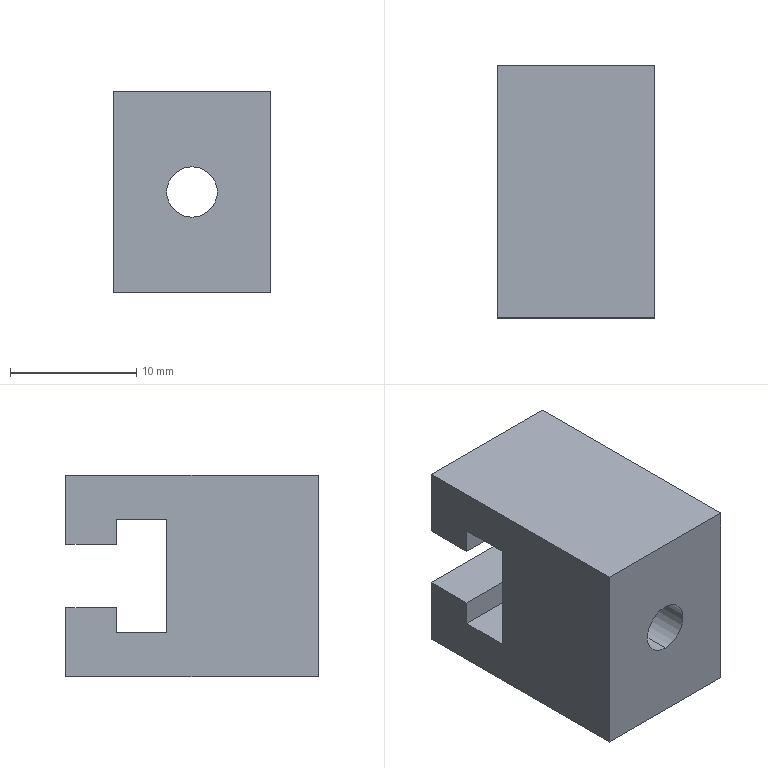Part | STEP file | 1 solid | 16 faces | box 12.5 x 20 x 16 mm | volume 3149 mm3 | plane 14 | cylinder 2 | commonest cylinder face diameters 4 x2
STEP:
#1=CARTESIAN_POINT('',(0.,0.,0.));
#2=DIRECTION('',(0.,0.,1.));
#3=DIRECTION('',(1.,0.,0.));
#4=AXIS2_PLACEMENT_3D('',#1,#2,#3);
#5=CARTESIAN_POINT('',(-97.105,-90.,104.07));
#6=VERTEX_POINT('',#5);
#7=CARTESIAN_POINT('',(-97.105,-78.,104.07));
#8=VERTEX_POINT('',#7);
#9=CARTESIAN_POINT('',(-97.105,-90.,104.07));
#10=DIRECTION('',(0.,1.,0.));
#11=VECTOR('',#10,1.);
#12=LINE('',#9,#11);
#13=CARTESIAN_POINT('',(-97.105,-90.,102.07));
#14=DIRECTION('',(0.,1.,0.));
#15=DIRECTION('',(0.,0.,1.));
#16=AXIS2_PLACEMENT_3D('',#13,#14,#15);
#17=CYLINDRICAL_SURFACE('',#16,2.);
#18=CARTESIAN_POINT('',(6.283,0.));
#19=DIRECTION('',(0.,1.));
#20=VECTOR('',#19,1.);
#21=LINE('',#18,#20);
#22=(GEOMETRIC_REPRESENTATION_CONTEXT(2)PARAMETRIC_REPRESENTATION_CONTEXT()REPRESENTATION_CONTEXT('',''));
#23=DEFINITIONAL_REPRESENTATION('',(#21),#22);
#24=PCURVE('',#17,#23);
#25=CARTESIAN_POINT('',(-97.105,-90.,102.07));
#26=DIRECTION('',(0.,1.,0.));
#27=DIRECTION('',(0.,0.,1.));
#28=AXIS2_PLACEMENT_3D('',#25,#26,#27);
#29=CYLINDRICAL_SURFACE('',#28,2.);
#30=CARTESIAN_POINT('',(0.,0.));
#31=DIRECTION('',(0.,1.));
#32=VECTOR('',#31,1.);
#33=LINE('',#30,#32);
#34=(GEOMETRIC_REPRESENTATION_CONTEXT(2)PARAMETRIC_REPRESENTATION_CONTEXT()REPRESENTATION_CONTEXT('',''));
#35=DEFINITIONAL_REPRESENTATION('',(#33),#34);
#36=PCURVE('',#29,#35);
#37=SURFACE_CURVE('',#12,(#24,#36),.PCURVE_S1.);
#38=EDGE_CURVE('',#6,#8,#37,.T.);
#39=ORIENTED_EDGE('',*,*,#38,.T.);
#40=CARTESIAN_POINT('',(-97.105,-78.,100.07));
#41=VERTEX_POINT('',#40);
#42=CARTESIAN_POINT('',(-97.105,-78.,102.07));
#43=DIRECTION('',(0.,1.,0.));
#44=DIRECTION('',(0.,0.,-1.));
#45=AXIS2_PLACEMENT_3D('',#42,#43,#44);
#46=CIRCLE('',#45,2.);
#47=CARTESIAN_POINT('',(3.142,12.));
#48=DIRECTION('',(1.,0.));
#49=VECTOR('',#48,1.);
#50=LINE('',#47,#49);
#51=(GEOMETRIC_REPRESENTATION_CONTEXT(2)PARAMETRIC_REPRESENTATION_CONTEXT()REPRESENTATION_CONTEXT('',''));
#52=DEFINITIONAL_REPRESENTATION('',(#50),#51);
#53=PCURVE('',#17,#52);
#54=CARTESIAN_POINT('',(-72.862,-78.,115.03));
#55=DIRECTION('',(0.,-1.,0.));
#56=DIRECTION('',(0.,0.,-1.));
#57=AXIS2_PLACEMENT_3D('',#54,#55,#56);
#58=PLANE('',#57);
#59=CARTESIAN_POINT('',(14.959,-24.242));
#60=CARTESIAN_POINT('',(14.959,-27.706));
#61=CARTESIAN_POINT('',(11.959,-25.974));
#62=CARTESIAN_POINT('',(8.959,-24.242));
#63=CARTESIAN_POINT('',(11.959,-22.51));
#64=CARTESIAN_POINT('',(14.959,-20.778));
#65=CARTESIAN_POINT('',(14.959,-24.242));
#66=(BOUNDED_CURVE()B_SPLINE_CURVE(2,(#59,#60,#61,#62,#63,#64,#65),.UNSPECIFIED.,.T.,.F.)B_SPLINE_CURVE_WITH_KNOTS((1,2,2,2,2,1),(-2.094,0.,2.094,4.189,6.283,8.378),.UNSPECIFIED.)CURVE()GEOMETRIC_REPRESENTATION_ITEM()RATIONAL_B_SPLINE_CURVE((1.,0.5,1.,0.5,1.,0.5,1.))REPRESENTATION_ITEM(''));
#67=(GEOMETRIC_REPRESENTATION_CONTEXT(2)PARAMETRIC_REPRESENTATION_CONTEXT()REPRESENTATION_CONTEXT('',''));
#68=DEFINITIONAL_REPRESENTATION('',(#66),#67);
#69=PCURVE('',#58,#68);
#70=SURFACE_CURVE('',#46,(#53,#69),.PCURVE_S1.);
#71=EDGE_CURVE('',#41,#8,#70,.T.);
#72=ORIENTED_EDGE('',*,*,#71,.F.);
#73=CARTESIAN_POINT('',(-97.105,-90.,100.07));
#74=VERTEX_POINT('',#73);
#75=CARTESIAN_POINT('',(-97.105,-90.,100.07));
#76=DIRECTION('',(0.,1.,0.));
#77=VECTOR('',#76,1.);
#78=LINE('',#75,#77);
#79=CARTESIAN_POINT('',(3.142,0.));
#80=DIRECTION('',(0.,1.));
#81=VECTOR('',#80,1.);
#82=LINE('',#79,#81);
#83=(GEOMETRIC_REPRESENTATION_CONTEXT(2)PARAMETRIC_REPRESENTATION_CONTEXT()REPRESENTATION_CONTEXT('',''));
#84=DEFINITIONAL_REPRESENTATION('',(#82),#83);
#85=PCURVE('',#17,#84);
#86=CARTESIAN_POINT('',(3.142,0.));
#87=DIRECTION('',(0.,1.));
#88=VECTOR('',#87,1.);
#89=LINE('',#86,#88);
#90=(GEOMETRIC_REPRESENTATION_CONTEXT(2)PARAMETRIC_REPRESENTATION_CONTEXT()REPRESENTATION_CONTEXT('',''));
#91=DEFINITIONAL_REPRESENTATION('',(#89),#90);
#92=PCURVE('',#29,#91);
#93=SURFACE_CURVE('',#78,(#85,#92),.PCURVE_S1.);
#94=EDGE_CURVE('',#74,#41,#93,.T.);
#95=ORIENTED_EDGE('',*,*,#94,.F.);
#96=CARTESIAN_POINT('',(-97.105,-90.,102.07));
#97=DIRECTION('',(0.,1.,0.));
#98=DIRECTION('',(0.,0.,1.));
#99=AXIS2_PLACEMENT_3D('',#96,#97,#98);
#100=CIRCLE('',#99,2.);
#101=CARTESIAN_POINT('',(0.,0.));
#102=DIRECTION('',(1.,0.));
#103=VECTOR('',#102,1.);
#104=LINE('',#101,#103);
#105=(GEOMETRIC_REPRESENTATION_CONTEXT(2)PARAMETRIC_REPRESENTATION_CONTEXT()REPRESENTATION_CONTEXT('',''));
#106=DEFINITIONAL_REPRESENTATION('',(#104),#105);
#107=PCURVE('',#17,#106);
#108=CARTESIAN_POINT('',(-96.957,-90.,94.07));
#109=DIRECTION('',(0.,-1.,0.));
#110=DIRECTION('',(0.,0.,-1.));
#111=AXIS2_PLACEMENT_3D('',#108,#109,#110);
#112=PLANE('',#111);
#113=CARTESIAN_POINT('',(-10.,-0.1474));
#114=CARTESIAN_POINT('',(-10.,3.317));
#115=CARTESIAN_POINT('',(-7.,1.585));
#116=CARTESIAN_POINT('',(-4.,-0.1474));
#117=CARTESIAN_POINT('',(-7.,-1.879));
#118=CARTESIAN_POINT('',(-10.,-3.612));
#119=CARTESIAN_POINT('',(-10.,-0.1474));
#120=(BOUNDED_CURVE()B_SPLINE_CURVE(2,(#113,#114,#115,#116,#117,#118,#119),.UNSPECIFIED.,.T.,.F.)B_SPLINE_CURVE_WITH_KNOTS((1,2,2,2,2,1),(-2.094,0.,2.094,4.189,6.283,8.378),.UNSPECIFIED.)CURVE()GEOMETRIC_REPRESENTATION_ITEM()RATIONAL_B_SPLINE_CURVE((1.,0.5,1.,0.5,1.,0.5,1.))REPRESENTATION_ITEM(''));
#121=(GEOMETRIC_REPRESENTATION_CONTEXT(2)PARAMETRIC_REPRESENTATION_CONTEXT()REPRESENTATION_CONTEXT('',''));
#122=DEFINITIONAL_REPRESENTATION('',(#120),#121);
#123=PCURVE('',#112,#122);
#124=SURFACE_CURVE('',#100,(#107,#123),.PCURVE_S1.);
#125=EDGE_CURVE('',#74,#6,#124,.T.);
#126=ORIENTED_EDGE('',*,*,#125,.T.);
#127=EDGE_LOOP('',(#39,#72,#95,#126));
#128=FACE_BOUND('',#127,.F.);
#129=ADVANCED_FACE('',(#128),#17,.F.);
#130=CARTESIAN_POINT('',(-103.355,-70.,104.57));
#131=VERTEX_POINT('',#130);
#132=CARTESIAN_POINT('',(-103.355,-70.,110.07));
#133=VERTEX_POINT('',#132);
#134=CARTESIAN_POINT('',(-103.355,-70.,94.07));
#135=DIRECTION('',(0.,0.,1.));
#136=VECTOR('',#135,1.);
#137=LINE('',#134,#136);
#138=CARTESIAN_POINT('',(-103.355,-85.,94.07));
#139=DIRECTION('',(-1.,0.,0.));
#140=DIRECTION('',(0.,0.,1.));
#141=AXIS2_PLACEMENT_3D('',#138,#139,#140);
#142=PLANE('',#141);
#143=CARTESIAN_POINT('',(0.,15.));
#144=DIRECTION('',(1.,0.));
#145=VECTOR('',#144,1.);
#146=LINE('',#143,#145);
#147=(GEOMETRIC_REPRESENTATION_CONTEXT(2)PARAMETRIC_REPRESENTATION_CONTEXT()REPRESENTATION_CONTEXT('',''));
#148=DEFINITIONAL_REPRESENTATION('',(#146),#147);
#149=PCURVE('',#142,#148);
#150=CARTESIAN_POINT('',(-96.957,-70.,94.07));
#151=DIRECTION('',(0.,1.,0.));
#152=DIRECTION('',(0.,0.,1.));
#153=AXIS2_PLACEMENT_3D('',#150,#151,#152);
#154=PLANE('',#153);
#155=CARTESIAN_POINT('',(0.,-6.397));
#156=DIRECTION('',(1.,0.));
#157=VECTOR('',#156,1.);
#158=LINE('',#155,#157);
#159=(GEOMETRIC_REPRESENTATION_CONTEXT(2)PARAMETRIC_REPRESENTATION_CONTEXT()REPRESENTATION_CONTEXT('',''));
#160=DEFINITIONAL_REPRESENTATION('',(#158),#159);
#161=PCURVE('',#154,#160);
#162=SURFACE_CURVE('',#137,(#149,#161),.PCURVE_S1.);
#163=EDGE_CURVE('',#131,#133,#162,.T.);
#164=ORIENTED_EDGE('',*,*,#163,.F.);
#165=CARTESIAN_POINT('',(-103.355,-74.,104.57));
#166=VERTEX_POINT('',#165);
#167=CARTESIAN_POINT('',(-103.355,-85.,104.57));
#168=DIRECTION('',(0.,-1.,0.));
#169=VECTOR('',#168,1.);
#170=LINE('',#167,#169);
#171=CARTESIAN_POINT('',(10.5,0.));
#172=DIRECTION('',(0.,-1.));
#173=VECTOR('',#172,1.);
#174=LINE('',#171,#173);
#175=(GEOMETRIC_REPRESENTATION_CONTEXT(2)PARAMETRIC_REPRESENTATION_CONTEXT()REPRESENTATION_CONTEXT('',''));
#176=DEFINITIONAL_REPRESENTATION('',(#174),#175);
#177=PCURVE('',#142,#176);
#178=CARTESIAN_POINT('',(-102.473,-26.188,104.57));
#179=DIRECTION('',(0.,0.,-1.));
#180=DIRECTION('',(-1.,0.,0.));
#181=AXIS2_PLACEMENT_3D('',#178,#179,#180);
#182=PLANE('',#181);
#183=CARTESIAN_POINT('',(0.8819,-58.812));
#184=DIRECTION('',(0.,-1.));
#185=VECTOR('',#184,1.);
#186=LINE('',#183,#185);
#187=(GEOMETRIC_REPRESENTATION_CONTEXT(2)PARAMETRIC_REPRESENTATION_CONTEXT()REPRESENTATION_CONTEXT('',''));
#188=DEFINITIONAL_REPRESENTATION('',(#186),#187);
#189=PCURVE('',#182,#188);
#190=SURFACE_CURVE('',#170,(#177,#189),.PCURVE_S1.);
#191=EDGE_CURVE('',#131,#166,#190,.T.);
#192=ORIENTED_EDGE('',*,*,#191,.T.);
#193=CARTESIAN_POINT('',(-103.355,-74.,106.57));
#194=VERTEX_POINT('',#193);
#195=CARTESIAN_POINT('',(-103.355,-74.,94.07));
#196=DIRECTION('',(0.,0.,1.));
#197=VECTOR('',#196,1.);
#198=LINE('',#195,#197);
#199=CARTESIAN_POINT('',(0.,11.));
#200=DIRECTION('',(1.,0.));
#201=VECTOR('',#200,1.);
#202=LINE('',#199,#201);
#203=(GEOMETRIC_REPRESENTATION_CONTEXT(2)PARAMETRIC_REPRESENTATION_CONTEXT()REPRESENTATION_CONTEXT('',''));
#204=DEFINITIONAL_REPRESENTATION('',(#202),#203);
#205=PCURVE('',#142,#204);
#206=CARTESIAN_POINT('',(-38.279,-74.,95.192));
#207=DIRECTION('',(0.,-1.,0.));
#208=DIRECTION('',(0.,0.,-1.));
#209=AXIS2_PLACEMENT_3D('',#206,#207,#208);
#210=PLANE('',#209);
#211=CARTESIAN_POINT('',(1.122,-65.076));
#212=DIRECTION('',(-1.,0.));
#213=VECTOR('',#212,1.);
#214=LINE('',#211,#213);
#215=(GEOMETRIC_REPRESENTATION_CONTEXT(2)PARAMETRIC_REPRESENTATION_CONTEXT()REPRESENTATION_CONTEXT('',''));
#216=DEFINITIONAL_REPRESENTATION('',(#214),#215);
#217=PCURVE('',#210,#216);
#218=SURFACE_CURVE('',#198,(#205,#217),.PCURVE_S1.);
#219=EDGE_CURVE('',#166,#194,#218,.T.);
#220=ORIENTED_EDGE('',*,*,#219,.T.);
#221=CARTESIAN_POINT('',(-103.355,-78.,106.57));
#222=VERTEX_POINT('',#221);
#223=CARTESIAN_POINT('',(-103.355,-85.,106.57));
#224=DIRECTION('',(0.,-1.,0.));
#225=VECTOR('',#224,1.);
#226=LINE('',#223,#225);
#227=CARTESIAN_POINT('',(12.5,0.));
#228=DIRECTION('',(0.,-1.));
#229=VECTOR('',#228,1.);
#230=LINE('',#227,#229);
#231=(GEOMETRIC_REPRESENTATION_CONTEXT(2)PARAMETRIC_REPRESENTATION_CONTEXT()REPRESENTATION_CONTEXT('',''));
#232=DEFINITIONAL_REPRESENTATION('',(#230),#231);
#233=PCURVE('',#142,#232);
#234=CARTESIAN_POINT('',(-102.473,-26.188,106.57));
#235=DIRECTION('',(0.,0.,-1.));
#236=DIRECTION('',(-1.,0.,0.));
#237=AXIS2_PLACEMENT_3D('',#234,#235,#236);
#238=PLANE('',#237);
#239=CARTESIAN_POINT('',(0.8819,-58.812));
#240=DIRECTION('',(0.,-1.));
#241=VECTOR('',#240,1.);
#242=LINE('',#239,#241);
#243=(GEOMETRIC_REPRESENTATION_CONTEXT(2)PARAMETRIC_REPRESENTATION_CONTEXT()REPRESENTATION_CONTEXT('',''));
#244=DEFINITIONAL_REPRESENTATION('',(#242),#243);
#245=PCURVE('',#238,#244);
#246=SURFACE_CURVE('',#226,(#233,#245),.PCURVE_S1.);
#247=EDGE_CURVE('',#194,#222,#246,.T.);
#248=ORIENTED_EDGE('',*,*,#247,.T.);
#249=CARTESIAN_POINT('',(-103.355,-78.,97.57));
#250=VERTEX_POINT('',#249);
#251=CARTESIAN_POINT('',(-103.355,-78.,94.07));
#252=DIRECTION('',(0.,0.,-1.));
#253=VECTOR('',#252,1.);
#254=LINE('',#251,#253);
#255=CARTESIAN_POINT('',(0.,7.));
#256=DIRECTION('',(-1.,0.));
#257=VECTOR('',#256,1.);
#258=LINE('',#255,#257);
#259=(GEOMETRIC_REPRESENTATION_CONTEXT(2)PARAMETRIC_REPRESENTATION_CONTEXT()REPRESENTATION_CONTEXT('',''));
#260=DEFINITIONAL_REPRESENTATION('',(#258),#259);
#261=PCURVE('',#142,#260);
#262=CARTESIAN_POINT('',(20.959,-30.492));
#263=DIRECTION('',(1.,0.));
#264=VECTOR('',#263,1.);
#265=LINE('',#262,#264);
#266=(GEOMETRIC_REPRESENTATION_CONTEXT(2)PARAMETRIC_REPRESENTATION_CONTEXT()REPRESENTATION_CONTEXT('',''));
#267=DEFINITIONAL_REPRESENTATION('',(#265),#266);
#268=PCURVE('',#58,#267);
#269=SURFACE_CURVE('',#254,(#261,#268),.PCURVE_S1.);
#270=EDGE_CURVE('',#222,#250,#269,.T.);
#271=ORIENTED_EDGE('',*,*,#270,.T.);
#272=CARTESIAN_POINT('',(-103.355,-74.,97.57));
#273=VERTEX_POINT('',#272);
#274=CARTESIAN_POINT('',(-103.355,-85.,97.57));
#275=DIRECTION('',(0.,1.,0.));
#276=VECTOR('',#275,1.);
#277=LINE('',#274,#276);
#278=CARTESIAN_POINT('',(3.5,0.));
#279=DIRECTION('',(0.,1.));
#280=VECTOR('',#279,1.);
#281=LINE('',#278,#280);
#282=(GEOMETRIC_REPRESENTATION_CONTEXT(2)PARAMETRIC_REPRESENTATION_CONTEXT()REPRESENTATION_CONTEXT('',''));
#283=DEFINITIONAL_REPRESENTATION('',(#281),#282);
#284=PCURVE('',#142,#283);
#285=CARTESIAN_POINT('',(-103.611,150.,97.57));
#286=DIRECTION('',(0.,0.,1.));
#287=DIRECTION('',(1.,0.,0.));
#288=AXIS2_PLACEMENT_3D('',#285,#286,#287);
#289=PLANE('',#288);
#290=CARTESIAN_POINT('',(0.2561,-235.));
#291=DIRECTION('',(0.,1.));
#292=VECTOR('',#291,1.);
#293=LINE('',#290,#292);
#294=(GEOMETRIC_REPRESENTATION_CONTEXT(2)PARAMETRIC_REPRESENTATION_CONTEXT()REPRESENTATION_CONTEXT('',''));
#295=DEFINITIONAL_REPRESENTATION('',(#293),#294);
#296=PCURVE('',#289,#295);
#297=SURFACE_CURVE('',#277,(#284,#296),.PCURVE_S1.);
#298=EDGE_CURVE('',#250,#273,#297,.T.);
#299=ORIENTED_EDGE('',*,*,#298,.T.);
#300=CARTESIAN_POINT('',(-103.355,-74.,99.57));
#301=VERTEX_POINT('',#300);
#302=CARTESIAN_POINT('',(-103.355,-74.,94.07));
#303=DIRECTION('',(0.,0.,1.));
#304=VECTOR('',#303,1.);
#305=LINE('',#302,#304);
#306=CARTESIAN_POINT('',(0.,11.));
#307=DIRECTION('',(1.,0.));
#308=VECTOR('',#307,1.);
#309=LINE('',#306,#308);
#310=(GEOMETRIC_REPRESENTATION_CONTEXT(2)PARAMETRIC_REPRESENTATION_CONTEXT()REPRESENTATION_CONTEXT('',''));
#311=DEFINITIONAL_REPRESENTATION('',(#309),#310);
#312=PCURVE('',#142,#311);
#313=CARTESIAN_POINT('',(-38.279,-74.,95.192));
#314=DIRECTION('',(0.,-1.,0.));
#315=DIRECTION('',(0.,0.,-1.));
#316=AXIS2_PLACEMENT_3D('',#313,#314,#315);
#317=PLANE('',#316);
#318=CARTESIAN_POINT('',(1.122,-65.076));
#319=DIRECTION('',(-1.,0.));
#320=VECTOR('',#319,1.);
#321=LINE('',#318,#320);
#322=(GEOMETRIC_REPRESENTATION_CONTEXT(2)PARAMETRIC_REPRESENTATION_CONTEXT()REPRESENTATION_CONTEXT('',''));
#323=DEFINITIONAL_REPRESENTATION('',(#321),#322);
#324=PCURVE('',#317,#323);
#325=SURFACE_CURVE('',#305,(#312,#324),.PCURVE_S1.);
#326=EDGE_CURVE('',#273,#301,#325,.T.);
#327=ORIENTED_EDGE('',*,*,#326,.T.);
#328=CARTESIAN_POINT('',(-103.355,-70.,99.57));
#329=VERTEX_POINT('',#328);
#330=CARTESIAN_POINT('',(-103.355,-85.,99.57));
#331=DIRECTION('',(0.,1.,0.));
#332=VECTOR('',#331,1.);
#333=LINE('',#330,#332);
#334=CARTESIAN_POINT('',(5.5,0.));
#335=DIRECTION('',(0.,1.));
#336=VECTOR('',#335,1.);
#337=LINE('',#334,#336);
#338=(GEOMETRIC_REPRESENTATION_CONTEXT(2)PARAMETRIC_REPRESENTATION_CONTEXT()REPRESENTATION_CONTEXT('',''));
#339=DEFINITIONAL_REPRESENTATION('',(#337),#338);
#340=PCURVE('',#142,#339);
#341=CARTESIAN_POINT('',(-103.611,150.,99.57));
#342=DIRECTION('',(0.,0.,1.));
#343=DIRECTION('',(1.,0.,0.));
#344=AXIS2_PLACEMENT_3D('',#341,#342,#343);
#345=PLANE('',#344);
#346=CARTESIAN_POINT('',(0.2561,-235.));
#347=DIRECTION('',(0.,1.));
#348=VECTOR('',#347,1.);
#349=LINE('',#346,#348);
#350=(GEOMETRIC_REPRESENTATION_CONTEXT(2)PARAMETRIC_REPRESENTATION_CONTEXT()REPRESENTATION_CONTEXT('',''));
#351=DEFINITIONAL_REPRESENTATION('',(#349),#350);
#352=PCURVE('',#345,#351);
#353=SURFACE_CURVE('',#333,(#340,#352),.PCURVE_S1.);
#354=EDGE_CURVE('',#301,#329,#353,.T.);
#355=ORIENTED_EDGE('',*,*,#354,.T.);
#356=CARTESIAN_POINT('',(-103.355,-70.,94.07));
#357=VERTEX_POINT('',#356);
#358=CARTESIAN_POINT('',(-103.355,-70.,94.07));
#359=DIRECTION('',(0.,0.,1.));
#360=VECTOR('',#359,1.);
#361=LINE('',#358,#360);
#362=CARTESIAN_POINT('',(0.,15.));
#363=DIRECTION('',(1.,0.));
#364=VECTOR('',#363,1.);
#365=LINE('',#362,#364);
#366=(GEOMETRIC_REPRESENTATION_CONTEXT(2)PARAMETRIC_REPRESENTATION_CONTEXT()REPRESENTATION_CONTEXT('',''));
#367=DEFINITIONAL_REPRESENTATION('',(#365),#366);
#368=PCURVE('',#142,#367);
#369=CARTESIAN_POINT('',(-96.957,-70.,94.07));
#370=DIRECTION('',(0.,1.,0.));
#371=DIRECTION('',(0.,0.,1.));
#372=AXIS2_PLACEMENT_3D('',#369,#370,#371);
#373=PLANE('',#372);
#374=CARTESIAN_POINT('',(0.,-6.397));
#375=DIRECTION('',(1.,0.));
#376=VECTOR('',#375,1.);
#377=LINE('',#374,#376);
#378=(GEOMETRIC_REPRESENTATION_CONTEXT(2)PARAMETRIC_REPRESENTATION_CONTEXT()REPRESENTATION_CONTEXT('',''));
#379=DEFINITIONAL_REPRESENTATION('',(#377),#378);
#380=PCURVE('',#373,#379);
#381=SURFACE_CURVE('',#361,(#368,#380),.PCURVE_S1.);
#382=EDGE_CURVE('',#357,#329,#381,.T.);
#383=ORIENTED_EDGE('',*,*,#382,.F.);
#384=CARTESIAN_POINT('',(-103.355,-90.,94.07));
#385=VERTEX_POINT('',#384);
#386=CARTESIAN_POINT('',(-103.355,-85.,94.07));
#387=DIRECTION('',(0.,-1.,0.));
#388=VECTOR('',#387,1.);
#389=LINE('',#386,#388);
#390=CARTESIAN_POINT('',(0.,0.));
#391=DIRECTION('',(0.,-1.));
#392=VECTOR('',#391,1.);
#393=LINE('',#390,#392);
#394=(GEOMETRIC_REPRESENTATION_CONTEXT(2)PARAMETRIC_REPRESENTATION_CONTEXT()REPRESENTATION_CONTEXT('',''));
#395=DEFINITIONAL_REPRESENTATION('',(#393),#394);
#396=PCURVE('',#142,#395);
#397=CARTESIAN_POINT('',(-96.957,-85.,94.07));
#398=DIRECTION('',(0.,0.,-1.));
#399=DIRECTION('',(-1.,0.,0.));
#400=AXIS2_PLACEMENT_3D('',#397,#398,#399);
#401=PLANE('',#400);
#402=CARTESIAN_POINT('',(6.397,0.));
#403=DIRECTION('',(0.,-1.));
#404=VECTOR('',#403,1.);
#405=LINE('',#402,#404);
#406=(GEOMETRIC_REPRESENTATION_CONTEXT(2)PARAMETRIC_REPRESENTATION_CONTEXT()REPRESENTATION_CONTEXT('',''));
#407=DEFINITIONAL_REPRESENTATION('',(#405),#406);
#408=PCURVE('',#401,#407);
#409=SURFACE_CURVE('',#389,(#396,#408),.PCURVE_S1.);
#410=EDGE_CURVE('',#357,#385,#409,.T.);
#411=ORIENTED_EDGE('',*,*,#410,.T.);
#412=CARTESIAN_POINT('',(-103.355,-90.,110.07));
#413=VERTEX_POINT('',#412);
#414=CARTESIAN_POINT('',(-103.355,-90.,94.07));
#415=DIRECTION('',(0.,0.,1.));
#416=VECTOR('',#415,1.);
#417=LINE('',#414,#416);
#418=CARTESIAN_POINT('',(0.,-5.));
#419=DIRECTION('',(1.,0.));
#420=VECTOR('',#419,1.);
#421=LINE('',#418,#420);
#422=(GEOMETRIC_REPRESENTATION_CONTEXT(2)PARAMETRIC_REPRESENTATION_CONTEXT()REPRESENTATION_CONTEXT('',''));
#423=DEFINITIONAL_REPRESENTATION('',(#421),#422);
#424=PCURVE('',#142,#423);
#425=CARTESIAN_POINT('',(0.,-6.397));
#426=DIRECTION('',(-1.,0.));
#427=VECTOR('',#426,1.);
#428=LINE('',#425,#427);
#429=(GEOMETRIC_REPRESENTATION_CONTEXT(2)PARAMETRIC_REPRESENTATION_CONTEXT()REPRESENTATION_CONTEXT('',''));
#430=DEFINITIONAL_REPRESENTATION('',(#428),#429);
#431=PCURVE('',#112,#430);
#432=SURFACE_CURVE('',#417,(#424,#431),.PCURVE_S1.);
#433=EDGE_CURVE('',#385,#413,#432,.T.);
#434=ORIENTED_EDGE('',*,*,#433,.T.);
#435=CARTESIAN_POINT('',(-103.355,-85.,110.07));
#436=DIRECTION('',(0.,1.,0.));
#437=VECTOR('',#436,1.);
#438=LINE('',#435,#437);
#439=CARTESIAN_POINT('',(16.,0.));
#440=DIRECTION('',(0.,1.));
#441=VECTOR('',#440,1.);
#442=LINE('',#439,#441);
#443=(GEOMETRIC_REPRESENTATION_CONTEXT(2)PARAMETRIC_REPRESENTATION_CONTEXT()REPRESENTATION_CONTEXT('',''));
#444=DEFINITIONAL_REPRESENTATION('',(#442),#443);
#445=PCURVE('',#142,#444);
#446=CARTESIAN_POINT('',(-96.957,-85.,110.07));
#447=DIRECTION('',(0.,0.,1.));
#448=DIRECTION('',(1.,0.,0.));
#449=AXIS2_PLACEMENT_3D('',#446,#447,#448);
#450=PLANE('',#449);
#451=CARTESIAN_POINT('',(-6.397,0.));
#452=DIRECTION('',(0.,1.));
#453=VECTOR('',#452,1.);
#454=LINE('',#451,#453);
#455=(GEOMETRIC_REPRESENTATION_CONTEXT(2)PARAMETRIC_REPRESENTATION_CONTEXT()REPRESENTATION_CONTEXT('',''));
#456=DEFINITIONAL_REPRESENTATION('',(#454),#455);
#457=PCURVE('',#450,#456);
#458=SURFACE_CURVE('',#438,(#445,#457),.PCURVE_S1.);
#459=EDGE_CURVE('',#413,#133,#458,.T.);
#460=ORIENTED_EDGE('',*,*,#459,.T.);
#461=EDGE_LOOP('',(#164,#192,#220,#248,#271,#299,#327,#355,#383,#411,#434,#460));
#462=FACE_BOUND('',#461,.T.);
#463=ADVANCED_FACE('',(#462),#142,.T.);
#464=CARTESIAN_POINT('',(-90.855,-70.,104.57));
#465=VERTEX_POINT('',#464);
#466=CARTESIAN_POINT('',(-90.855,-70.,110.07));
#467=VERTEX_POINT('',#466);
#468=CARTESIAN_POINT('',(-90.855,-70.,94.07));
#469=DIRECTION('',(0.,0.,1.));
#470=VECTOR('',#469,1.);
#471=LINE('',#468,#470);
#472=CARTESIAN_POINT('',(0.,6.103));
#473=DIRECTION('',(1.,0.));
#474=VECTOR('',#473,1.);
#475=LINE('',#472,#474);
#476=(GEOMETRIC_REPRESENTATION_CONTEXT(2)PARAMETRIC_REPRESENTATION_CONTEXT()REPRESENTATION_CONTEXT('',''));
#477=DEFINITIONAL_REPRESENTATION('',(#475),#476);
#478=PCURVE('',#154,#477);
#479=CARTESIAN_POINT('',(-90.855,-80.,102.07));
#480=DIRECTION('',(-1.,0.,0.));
#481=DIRECTION('',(0.,0.,1.));
#482=AXIS2_PLACEMENT_3D('',#479,#480,#481);
#483=PLANE('',#482);
#484=CARTESIAN_POINT('',(-8.,10.));
#485=DIRECTION('',(1.,0.));
#486=VECTOR('',#485,1.);
#487=LINE('',#484,#486);
#488=(GEOMETRIC_REPRESENTATION_CONTEXT(2)PARAMETRIC_REPRESENTATION_CONTEXT()REPRESENTATION_CONTEXT('',''));
#489=DEFINITIONAL_REPRESENTATION('',(#487),#488);
#490=PCURVE('',#483,#489);
#491=SURFACE_CURVE('',#471,(#478,#490),.PCURVE_S1.);
#492=EDGE_CURVE('',#465,#467,#491,.T.);
#493=ORIENTED_EDGE('',*,*,#492,.F.);
#494=CARTESIAN_POINT('',(-96.957,-70.,104.57));
#495=DIRECTION('',(-1.,0.,0.));
#496=VECTOR('',#495,1.);
#497=LINE('',#494,#496);
#498=CARTESIAN_POINT('',(10.5,0.));
#499=DIRECTION('',(0.,-1.));
#500=VECTOR('',#499,1.);
#501=LINE('',#498,#500);
#502=(GEOMETRIC_REPRESENTATION_CONTEXT(2)PARAMETRIC_REPRESENTATION_CONTEXT()REPRESENTATION_CONTEXT('',''));
#503=DEFINITIONAL_REPRESENTATION('',(#501),#502);
#504=PCURVE('',#154,#503);
#505=CARTESIAN_POINT('',(-5.516,-43.812));
#506=DIRECTION('',(1.,0.));
#507=VECTOR('',#506,1.);
#508=LINE('',#505,#507);
#509=(GEOMETRIC_REPRESENTATION_CONTEXT(2)PARAMETRIC_REPRESENTATION_CONTEXT()REPRESENTATION_CONTEXT('',''));
#510=DEFINITIONAL_REPRESENTATION('',(#508),#509);
#511=PCURVE('',#182,#510);
#512=SURFACE_CURVE('',#497,(#504,#511),.PCURVE_S1.);
#513=EDGE_CURVE('',#465,#131,#512,.T.);
#514=ORIENTED_EDGE('',*,*,#513,.T.);
#515=ORIENTED_EDGE('',*,*,#163,.T.);
#516=CARTESIAN_POINT('',(-96.957,-70.,110.07));
#517=DIRECTION('',(1.,0.,0.));
#518=VECTOR('',#517,1.);
#519=LINE('',#516,#518);
#520=CARTESIAN_POINT('',(16.,0.));
#521=DIRECTION('',(0.,1.));
#522=VECTOR('',#521,1.);
#523=LINE('',#520,#522);
#524=(GEOMETRIC_REPRESENTATION_CONTEXT(2)PARAMETRIC_REPRESENTATION_CONTEXT()REPRESENTATION_CONTEXT('',''));
#525=DEFINITIONAL_REPRESENTATION('',(#523),#524);
#526=PCURVE('',#154,#525);
#527=CARTESIAN_POINT('',(0.,15.));
#528=DIRECTION('',(1.,0.));
#529=VECTOR('',#528,1.);
#530=LINE('',#527,#529);
#531=(GEOMETRIC_REPRESENTATION_CONTEXT(2)PARAMETRIC_REPRESENTATION_CONTEXT()REPRESENTATION_CONTEXT('',''));
#532=DEFINITIONAL_REPRESENTATION('',(#530),#531);
#533=PCURVE('',#450,#532);
#534=SURFACE_CURVE('',#519,(#526,#533),.PCURVE_S1.);
#535=EDGE_CURVE('',#133,#467,#534,.T.);
#536=ORIENTED_EDGE('',*,*,#535,.T.);
#537=EDGE_LOOP('',(#493,#514,#515,#536));
#538=FACE_BOUND('',#537,.T.);
#539=ADVANCED_FACE('',(#538),#154,.T.);
#540=CARTESIAN_POINT('',(-90.855,-70.,94.07));
#541=VERTEX_POINT('',#540);
#542=CARTESIAN_POINT('',(-90.855,-70.,99.57));
#543=VERTEX_POINT('',#542);
#544=CARTESIAN_POINT('',(-90.855,-70.,94.07));
#545=DIRECTION('',(0.,0.,1.));
#546=VECTOR('',#545,1.);
#547=LINE('',#544,#546);
#548=CARTESIAN_POINT('',(0.,6.103));
#549=DIRECTION('',(1.,0.));
#550=VECTOR('',#549,1.);
#551=LINE('',#548,#550);
#552=(GEOMETRIC_REPRESENTATION_CONTEXT(2)PARAMETRIC_REPRESENTATION_CONTEXT()REPRESENTATION_CONTEXT('',''));
#553=DEFINITIONAL_REPRESENTATION('',(#551),#552);
#554=PCURVE('',#373,#553);
#555=CARTESIAN_POINT('',(-8.,10.));
#556=DIRECTION('',(1.,0.));
#557=VECTOR('',#556,1.);
#558=LINE('',#555,#557);
#559=(GEOMETRIC_REPRESENTATION_CONTEXT(2)PARAMETRIC_REPRESENTATION_CONTEXT()REPRESENTATION_CONTEXT('',''));
#560=DEFINITIONAL_REPRESENTATION('',(#558),#559);
#561=PCURVE('',#483,#560);
#562=SURFACE_CURVE('',#547,(#554,#561),.PCURVE_S1.);
#563=EDGE_CURVE('',#541,#543,#562,.T.);
#564=ORIENTED_EDGE('',*,*,#563,.F.);
#565=CARTESIAN_POINT('',(-96.957,-70.,94.07));
#566=DIRECTION('',(-1.,0.,0.));
#567=VECTOR('',#566,1.);
#568=LINE('',#565,#567);
#569=CARTESIAN_POINT('',(0.,0.));
#570=DIRECTION('',(0.,-1.));
#571=VECTOR('',#570,1.);
#572=LINE('',#569,#571);
#573=(GEOMETRIC_REPRESENTATION_CONTEXT(2)PARAMETRIC_REPRESENTATION_CONTEXT()REPRESENTATION_CONTEXT('',''));
#574=DEFINITIONAL_REPRESENTATION('',(#572),#573);
#575=PCURVE('',#373,#574);
#576=CARTESIAN_POINT('',(0.,15.));
#577=DIRECTION('',(1.,0.));
#578=VECTOR('',#577,1.);
#579=LINE('',#576,#578);
#580=(GEOMETRIC_REPRESENTATION_CONTEXT(2)PARAMETRIC_REPRESENTATION_CONTEXT()REPRESENTATION_CONTEXT('',''));
#581=DEFINITIONAL_REPRESENTATION('',(#579),#580);
#582=PCURVE('',#401,#581);
#583=SURFACE_CURVE('',#568,(#575,#582),.PCURVE_S1.);
#584=EDGE_CURVE('',#541,#357,#583,.T.);
#585=ORIENTED_EDGE('',*,*,#584,.T.);
#586=ORIENTED_EDGE('',*,*,#382,.T.);
#587=CARTESIAN_POINT('',(-96.957,-70.,99.57));
#588=DIRECTION('',(1.,0.,0.));
#589=VECTOR('',#588,1.);
#590=LINE('',#587,#589);
#591=CARTESIAN_POINT('',(5.5,0.));
#592=DIRECTION('',(0.,1.));
#593=VECTOR('',#592,1.);
#594=LINE('',#591,#593);
#595=(GEOMETRIC_REPRESENTATION_CONTEXT(2)PARAMETRIC_REPRESENTATION_CONTEXT()REPRESENTATION_CONTEXT('',''));
#596=DEFINITIONAL_REPRESENTATION('',(#594),#595);
#597=PCURVE('',#373,#596);
#598=CARTESIAN_POINT('',(6.654,-220.));
#599=DIRECTION('',(1.,0.));
#600=VECTOR('',#599,1.);
#601=LINE('',#598,#600);
#602=(GEOMETRIC_REPRESENTATION_CONTEXT(2)PARAMETRIC_REPRESENTATION_CONTEXT()REPRESENTATION_CONTEXT('',''));
#603=DEFINITIONAL_REPRESENTATION('',(#601),#602);
#604=PCURVE('',#345,#603);
#605=SURFACE_CURVE('',#590,(#597,#604),.PCURVE_S1.);
#606=EDGE_CURVE('',#329,#543,#605,.T.);
#607=ORIENTED_EDGE('',*,*,#606,.T.);
#608=EDGE_LOOP('',(#564,#585,#586,#607));
#609=FACE_BOUND('',#608,.T.);
#610=ADVANCED_FACE('',(#609),#373,.T.);
#611=CARTESIAN_POINT('',(-90.855,-90.,110.07));
#612=VERTEX_POINT('',#611);
#613=CARTESIAN_POINT('',(-90.855,-85.,110.07));
#614=DIRECTION('',(0.,-1.,0.));
#615=VECTOR('',#614,1.);
#616=LINE('',#613,#615);
#617=CARTESIAN_POINT('',(6.103,0.));
#618=DIRECTION('',(0.,-1.));
#619=VECTOR('',#618,1.);
#620=LINE('',#617,#619);
#621=(GEOMETRIC_REPRESENTATION_CONTEXT(2)PARAMETRIC_REPRESENTATION_CONTEXT()REPRESENTATION_CONTEXT('',''));
#622=DEFINITIONAL_REPRESENTATION('',(#620),#621);
#623=PCURVE('',#450,#622);
#624=CARTESIAN_POINT('',(8.,-5.));
#625=DIRECTION('',(0.,-1.));
#626=VECTOR('',#625,1.);
#627=LINE('',#624,#626);
#628=(GEOMETRIC_REPRESENTATION_CONTEXT(2)PARAMETRIC_REPRESENTATION_CONTEXT()REPRESENTATION_CONTEXT('',''));
#629=DEFINITIONAL_REPRESENTATION('',(#627),#628);
#630=PCURVE('',#483,#629);
#631=SURFACE_CURVE('',#616,(#623,#630),.PCURVE_S1.);
#632=EDGE_CURVE('',#467,#612,#631,.T.);
#633=ORIENTED_EDGE('',*,*,#632,.F.);
#634=ORIENTED_EDGE('',*,*,#535,.F.);
#635=ORIENTED_EDGE('',*,*,#459,.F.);
#636=CARTESIAN_POINT('',(-96.957,-90.,110.07));
#637=DIRECTION('',(-1.,0.,0.));
#638=VECTOR('',#637,1.);
#639=LINE('',#636,#638);
#640=CARTESIAN_POINT('',(0.,-5.));
#641=DIRECTION('',(-1.,0.));
#642=VECTOR('',#641,1.);
#643=LINE('',#640,#642);
#644=(GEOMETRIC_REPRESENTATION_CONTEXT(2)PARAMETRIC_REPRESENTATION_CONTEXT()REPRESENTATION_CONTEXT('',''));
#645=DEFINITIONAL_REPRESENTATION('',(#643),#644);
#646=PCURVE('',#450,#645);
#647=CARTESIAN_POINT('',(-16.,0.));
#648=DIRECTION('',(0.,-1.));
#649=VECTOR('',#648,1.);
#650=LINE('',#647,#649);
#651=(GEOMETRIC_REPRESENTATION_CONTEXT(2)PARAMETRIC_REPRESENTATION_CONTEXT()REPRESENTATION_CONTEXT('',''));
#652=DEFINITIONAL_REPRESENTATION('',(#650),#651);
#653=PCURVE('',#112,#652);
#654=SURFACE_CURVE('',#639,(#646,#653),.PCURVE_S1.);
#655=EDGE_CURVE('',#612,#413,#654,.T.);
#656=ORIENTED_EDGE('',*,*,#655,.F.);
#657=EDGE_LOOP('',(#633,#634,#635,#656));
#658=FACE_BOUND('',#657,.T.);
#659=ADVANCED_FACE('',(#658),#450,.T.);
#660=CARTESIAN_POINT('',(-97.105,-90.,102.07));
#661=DIRECTION('',(0.,1.,0.));
#662=DIRECTION('',(0.,0.,1.));
#663=AXIS2_PLACEMENT_3D('',#660,#661,#662);
#664=CIRCLE('',#663,2.);
#665=CARTESIAN_POINT('',(-10.,-0.1474));
#666=CARTESIAN_POINT('',(-10.,3.317));
#667=CARTESIAN_POINT('',(-7.,1.585));
#668=CARTESIAN_POINT('',(-4.,-0.1474));
#669=CARTESIAN_POINT('',(-7.,-1.879));
#670=CARTESIAN_POINT('',(-10.,-3.612));
#671=CARTESIAN_POINT('',(-10.,-0.1474));
#672=(BOUNDED_CURVE()B_SPLINE_CURVE(2,(#665,#666,#667,#668,#669,#670,#671),.UNSPECIFIED.,.T.,.F.)B_SPLINE_CURVE_WITH_KNOTS((1,2,2,2,2,1),(-2.094,0.,2.094,4.189,6.283,8.378),.UNSPECIFIED.)CURVE()GEOMETRIC_REPRESENTATION_ITEM()RATIONAL_B_SPLINE_CURVE((1.,0.5,1.,0.5,1.,0.5,1.))REPRESENTATION_ITEM(''));
#673=(GEOMETRIC_REPRESENTATION_CONTEXT(2)PARAMETRIC_REPRESENTATION_CONTEXT()REPRESENTATION_CONTEXT('',''));
#674=DEFINITIONAL_REPRESENTATION('',(#672),#673);
#675=PCURVE('',#112,#674);
#676=CARTESIAN_POINT('',(0.,0.));
#677=DIRECTION('',(1.,0.));
#678=VECTOR('',#677,1.);
#679=LINE('',#676,#678);
#680=(GEOMETRIC_REPRESENTATION_CONTEXT(2)PARAMETRIC_REPRESENTATION_CONTEXT()REPRESENTATION_CONTEXT('',''));
#681=DEFINITIONAL_REPRESENTATION('',(#679),#680);
#682=PCURVE('',#29,#681);
#683=SURFACE_CURVE('',#664,(#675,#682),.PCURVE_S1.);
#684=EDGE_CURVE('',#6,#74,#683,.T.);
#685=ORIENTED_EDGE('',*,*,#684,.T.);
#686=ORIENTED_EDGE('',*,*,#125,.T.);
#687=EDGE_LOOP('',(#685,#686));
#688=FACE_BOUND('',#687,.T.);
#689=CARTESIAN_POINT('',(-90.855,-90.,94.07));
#690=VERTEX_POINT('',#689);
#691=CARTESIAN_POINT('',(-90.855,-90.,94.07));
#692=DIRECTION('',(0.,0.,-1.));
#693=VECTOR('',#692,1.);
#694=LINE('',#691,#693);
#695=CARTESIAN_POINT('',(0.,6.103));
#696=DIRECTION('',(1.,0.));
#697=VECTOR('',#696,1.);
#698=LINE('',#695,#697);
#699=(GEOMETRIC_REPRESENTATION_CONTEXT(2)PARAMETRIC_REPRESENTATION_CONTEXT()REPRESENTATION_CONTEXT('',''));
#700=DEFINITIONAL_REPRESENTATION('',(#698),#699);
#701=PCURVE('',#112,#700);
#702=CARTESIAN_POINT('',(-8.,-10.));
#703=DIRECTION('',(-1.,0.));
#704=VECTOR('',#703,1.);
#705=LINE('',#702,#704);
#706=(GEOMETRIC_REPRESENTATION_CONTEXT(2)PARAMETRIC_REPRESENTATION_CONTEXT()REPRESENTATION_CONTEXT('',''));
#707=DEFINITIONAL_REPRESENTATION('',(#705),#706);
#708=PCURVE('',#483,#707);
#709=SURFACE_CURVE('',#694,(#701,#708),.PCURVE_S1.);
#710=EDGE_CURVE('',#612,#690,#709,.T.);
#711=ORIENTED_EDGE('',*,*,#710,.F.);
#712=ORIENTED_EDGE('',*,*,#655,.T.);
#713=ORIENTED_EDGE('',*,*,#433,.F.);
#714=CARTESIAN_POINT('',(-96.957,-90.,94.07));
#715=DIRECTION('',(1.,0.,0.));
#716=VECTOR('',#715,1.);
#717=LINE('',#714,#716);
#718=CARTESIAN_POINT('',(0.,0.));
#719=DIRECTION('',(0.,1.));
#720=VECTOR('',#719,1.);
#721=LINE('',#718,#720);
#722=(GEOMETRIC_REPRESENTATION_CONTEXT(2)PARAMETRIC_REPRESENTATION_CONTEXT()REPRESENTATION_CONTEXT('',''));
#723=DEFINITIONAL_REPRESENTATION('',(#721),#722);
#724=PCURVE('',#112,#723);
#725=CARTESIAN_POINT('',(0.,-5.));
#726=DIRECTION('',(-1.,0.));
#727=VECTOR('',#726,1.);
#728=LINE('',#725,#727);
#729=(GEOMETRIC_REPRESENTATION_CONTEXT(2)PARAMETRIC_REPRESENTATION_CONTEXT()REPRESENTATION_CONTEXT('',''));
#730=DEFINITIONAL_REPRESENTATION('',(#728),#729);
#731=PCURVE('',#401,#730);
#732=SURFACE_CURVE('',#717,(#724,#731),.PCURVE_S1.);
#733=EDGE_CURVE('',#385,#690,#732,.T.);
#734=ORIENTED_EDGE('',*,*,#733,.T.);
#735=EDGE_LOOP('',(#711,#712,#713,#734));
#736=FACE_BOUND('',#735,.T.);
#737=ADVANCED_FACE('',(#688,#736),#112,.T.);
#738=CARTESIAN_POINT('',(-90.855,-85.,94.07));
#739=DIRECTION('',(0.,1.,0.));
#740=VECTOR('',#739,1.);
#741=LINE('',#738,#740);
#742=CARTESIAN_POINT('',(-6.103,0.));
#743=DIRECTION('',(0.,1.));
#744=VECTOR('',#743,1.);
#745=LINE('',#742,#744);
#746=(GEOMETRIC_REPRESENTATION_CONTEXT(2)PARAMETRIC_REPRESENTATION_CONTEXT()REPRESENTATION_CONTEXT('',''));
#747=DEFINITIONAL_REPRESENTATION('',(#745),#746);
#748=PCURVE('',#401,#747);
#749=CARTESIAN_POINT('',(-8.,-5.));
#750=DIRECTION('',(0.,1.));
#751=VECTOR('',#750,1.);
#752=LINE('',#749,#751);
#753=(GEOMETRIC_REPRESENTATION_CONTEXT(2)PARAMETRIC_REPRESENTATION_CONTEXT()REPRESENTATION_CONTEXT('',''));
#754=DEFINITIONAL_REPRESENTATION('',(#752),#753);
#755=PCURVE('',#483,#754);
#756=SURFACE_CURVE('',#741,(#748,#755),.PCURVE_S1.);
#757=EDGE_CURVE('',#690,#541,#756,.T.);
#758=ORIENTED_EDGE('',*,*,#757,.F.);
#759=ORIENTED_EDGE('',*,*,#733,.F.);
#760=ORIENTED_EDGE('',*,*,#410,.F.);
#761=ORIENTED_EDGE('',*,*,#584,.F.);
#762=EDGE_LOOP('',(#758,#759,#760,#761));
#763=FACE_BOUND('',#762,.T.);
#764=ADVANCED_FACE('',(#763),#401,.T.);
#765=CARTESIAN_POINT('',(-90.855,-74.,106.57));
#766=VERTEX_POINT('',#765);
#767=CARTESIAN_POINT('',(-90.855,-74.,104.57));
#768=VERTEX_POINT('',#767);
#769=CARTESIAN_POINT('',(-90.855,-74.,95.192));
#770=DIRECTION('',(0.,0.,-1.));
#771=VECTOR('',#770,1.);
#772=LINE('',#769,#771);
#773=CARTESIAN_POINT('',(0.,-52.576));
#774=DIRECTION('',(1.,0.));
#775=VECTOR('',#774,1.);
#776=LINE('',#773,#775);
#777=(GEOMETRIC_REPRESENTATION_CONTEXT(2)PARAMETRIC_REPRESENTATION_CONTEXT()REPRESENTATION_CONTEXT('',''));
#778=DEFINITIONAL_REPRESENTATION('',(#776),#777);
#779=PCURVE('',#210,#778);
#780=CARTESIAN_POINT('',(-6.878,6.));
#781=DIRECTION('',(-1.,0.));
#782=VECTOR('',#781,1.);
#783=LINE('',#780,#782);
#784=(GEOMETRIC_REPRESENTATION_CONTEXT(2)PARAMETRIC_REPRESENTATION_CONTEXT()REPRESENTATION_CONTEXT('',''));
#785=DEFINITIONAL_REPRESENTATION('',(#783),#784);
#786=PCURVE('',#483,#785);
#787=SURFACE_CURVE('',#772,(#779,#786),.PCURVE_S1.);
#788=EDGE_CURVE('',#766,#768,#787,.T.);
#789=ORIENTED_EDGE('',*,*,#788,.F.);
#790=CARTESIAN_POINT('',(-102.473,-74.,106.57));
#791=DIRECTION('',(-1.,0.,0.));
#792=VECTOR('',#791,1.);
#793=LINE('',#790,#792);
#794=CARTESIAN_POINT('',(-11.378,-64.194));
#795=DIRECTION('',(0.,-1.));
#796=VECTOR('',#795,1.);
#797=LINE('',#794,#796);
#798=(GEOMETRIC_REPRESENTATION_CONTEXT(2)PARAMETRIC_REPRESENTATION_CONTEXT()REPRESENTATION_CONTEXT('',''));
#799=DEFINITIONAL_REPRESENTATION('',(#797),#798);
#800=PCURVE('',#210,#799);
#801=CARTESIAN_POINT('',(0.,-47.812));
#802=DIRECTION('',(1.,0.));
#803=VECTOR('',#802,1.);
#804=LINE('',#801,#803);
#805=(GEOMETRIC_REPRESENTATION_CONTEXT(2)PARAMETRIC_REPRESENTATION_CONTEXT()REPRESENTATION_CONTEXT('',''));
#806=DEFINITIONAL_REPRESENTATION('',(#804),#805);
#807=PCURVE('',#238,#806);
#808=SURFACE_CURVE('',#793,(#800,#807),.PCURVE_S1.);
#809=EDGE_CURVE('',#766,#194,#808,.T.);
#810=ORIENTED_EDGE('',*,*,#809,.T.);
#811=ORIENTED_EDGE('',*,*,#219,.F.);
#812=CARTESIAN_POINT('',(-102.473,-74.,104.57));
#813=DIRECTION('',(-1.,0.,0.));
#814=VECTOR('',#813,1.);
#815=LINE('',#812,#814);
#816=CARTESIAN_POINT('',(-9.378,-64.194));
#817=DIRECTION('',(0.,-1.));
#818=VECTOR('',#817,1.);
#819=LINE('',#816,#818);
#820=(GEOMETRIC_REPRESENTATION_CONTEXT(2)PARAMETRIC_REPRESENTATION_CONTEXT()REPRESENTATION_CONTEXT('',''));
#821=DEFINITIONAL_REPRESENTATION('',(#819),#820);
#822=PCURVE('',#210,#821);
#823=CARTESIAN_POINT('',(0.,-47.812));
#824=DIRECTION('',(1.,0.));
#825=VECTOR('',#824,1.);
#826=LINE('',#823,#825);
#827=(GEOMETRIC_REPRESENTATION_CONTEXT(2)PARAMETRIC_REPRESENTATION_CONTEXT()REPRESENTATION_CONTEXT('',''));
#828=DEFINITIONAL_REPRESENTATION('',(#826),#827);
#829=PCURVE('',#182,#828);
#830=SURFACE_CURVE('',#815,(#822,#829),.PCURVE_S1.);
#831=EDGE_CURVE('',#768,#166,#830,.T.);
#832=ORIENTED_EDGE('',*,*,#831,.F.);
#833=EDGE_LOOP('',(#789,#810,#811,#832));
#834=FACE_BOUND('',#833,.T.);
#835=ADVANCED_FACE('',(#834),#210,.T.);
#836=CARTESIAN_POINT('',(-97.105,-78.,102.07));
#837=DIRECTION('',(0.,1.,0.));
#838=DIRECTION('',(0.,0.,-1.));
#839=AXIS2_PLACEMENT_3D('',#836,#837,#838);
#840=CIRCLE('',#839,2.);
#841=CARTESIAN_POINT('',(14.959,-24.242));
#842=CARTESIAN_POINT('',(14.959,-27.706));
#843=CARTESIAN_POINT('',(11.959,-25.974));
#844=CARTESIAN_POINT('',(8.959,-24.242));
#845=CARTESIAN_POINT('',(11.959,-22.51));
#846=CARTESIAN_POINT('',(14.959,-20.778));
#847=CARTESIAN_POINT('',(14.959,-24.242));
#848=(BOUNDED_CURVE()B_SPLINE_CURVE(2,(#841,#842,#843,#844,#845,#846,#847),.UNSPECIFIED.,.T.,.F.)B_SPLINE_CURVE_WITH_KNOTS((1,2,2,2,2,1),(-2.094,0.,2.094,4.189,6.283,8.378),.UNSPECIFIED.)CURVE()GEOMETRIC_REPRESENTATION_ITEM()RATIONAL_B_SPLINE_CURVE((1.,0.5,1.,0.5,1.,0.5,1.))REPRESENTATION_ITEM(''));
#849=(GEOMETRIC_REPRESENTATION_CONTEXT(2)PARAMETRIC_REPRESENTATION_CONTEXT()REPRESENTATION_CONTEXT('',''));
#850=DEFINITIONAL_REPRESENTATION('',(#848),#849);
#851=PCURVE('',#58,#850);
#852=CARTESIAN_POINT('',(-3.142,12.));
#853=DIRECTION('',(1.,0.));
#854=VECTOR('',#853,1.);
#855=LINE('',#852,#854);
#856=(GEOMETRIC_REPRESENTATION_CONTEXT(2)PARAMETRIC_REPRESENTATION_CONTEXT()REPRESENTATION_CONTEXT('',''));
#857=DEFINITIONAL_REPRESENTATION('',(#855),#856);
#858=PCURVE('',#29,#857);
#859=SURFACE_CURVE('',#840,(#851,#858),.PCURVE_S1.);
#860=EDGE_CURVE('',#8,#41,#859,.T.);
#861=ORIENTED_EDGE('',*,*,#860,.F.);
#862=ORIENTED_EDGE('',*,*,#71,.F.);
#863=EDGE_LOOP('',(#861,#862));
#864=FACE_BOUND('',#863,.T.);
#865=CARTESIAN_POINT('',(-90.855,-78.,97.57));
#866=VERTEX_POINT('',#865);
#867=CARTESIAN_POINT('',(-90.855,-78.,106.57));
#868=VERTEX_POINT('',#867);
#869=CARTESIAN_POINT('',(-90.855,-78.,115.03));
#870=DIRECTION('',(0.,0.,1.));
#871=VECTOR('',#870,1.);
#872=LINE('',#869,#871);
#873=CARTESIAN_POINT('',(0.,-17.992));
#874=DIRECTION('',(-1.,0.));
#875=VECTOR('',#874,1.);
#876=LINE('',#873,#875);
#877=(GEOMETRIC_REPRESENTATION_CONTEXT(2)PARAMETRIC_REPRESENTATION_CONTEXT()REPRESENTATION_CONTEXT('',''));
#878=DEFINITIONAL_REPRESENTATION('',(#876),#877);
#879=PCURVE('',#58,#878);
#880=CARTESIAN_POINT('',(12.959,2.));
#881=DIRECTION('',(1.,0.));
#882=VECTOR('',#881,1.);
#883=LINE('',#880,#882);
#884=(GEOMETRIC_REPRESENTATION_CONTEXT(2)PARAMETRIC_REPRESENTATION_CONTEXT()REPRESENTATION_CONTEXT('',''));
#885=DEFINITIONAL_REPRESENTATION('',(#883),#884);
#886=PCURVE('',#483,#885);
#887=SURFACE_CURVE('',#872,(#879,#886),.PCURVE_S1.);
#888=EDGE_CURVE('',#866,#868,#887,.T.);
#889=ORIENTED_EDGE('',*,*,#888,.F.);
#890=CARTESIAN_POINT('',(-103.611,-78.,97.57));
#891=DIRECTION('',(-1.,0.,0.));
#892=VECTOR('',#891,1.);
#893=LINE('',#890,#892);
#894=CARTESIAN_POINT('',(17.459,-30.748));
#895=DIRECTION('',(0.,-1.));
#896=VECTOR('',#895,1.);
#897=LINE('',#894,#896);
#898=(GEOMETRIC_REPRESENTATION_CONTEXT(2)PARAMETRIC_REPRESENTATION_CONTEXT()REPRESENTATION_CONTEXT('',''));
#899=DEFINITIONAL_REPRESENTATION('',(#897),#898);
#900=PCURVE('',#58,#899);
#901=CARTESIAN_POINT('',(0.,-228.));
#902=DIRECTION('',(-1.,0.));
#903=VECTOR('',#902,1.);
#904=LINE('',#901,#903);
#905=(GEOMETRIC_REPRESENTATION_CONTEXT(2)PARAMETRIC_REPRESENTATION_CONTEXT()REPRESENTATION_CONTEXT('',''));
#906=DEFINITIONAL_REPRESENTATION('',(#904),#905);
#907=PCURVE('',#289,#906);
#908=SURFACE_CURVE('',#893,(#900,#907),.PCURVE_S1.);
#909=EDGE_CURVE('',#866,#250,#908,.T.);
#910=ORIENTED_EDGE('',*,*,#909,.T.);
#911=ORIENTED_EDGE('',*,*,#270,.F.);
#912=CARTESIAN_POINT('',(-72.862,-78.,106.57));
#913=DIRECTION('',(-1.,0.,0.));
#914=VECTOR('',#913,1.);
#915=LINE('',#912,#914);
#916=CARTESIAN_POINT('',(8.459,0.));
#917=DIRECTION('',(0.,-1.));
#918=VECTOR('',#917,1.);
#919=LINE('',#916,#918);
#920=(GEOMETRIC_REPRESENTATION_CONTEXT(2)PARAMETRIC_REPRESENTATION_CONTEXT()REPRESENTATION_CONTEXT('',''));
#921=DEFINITIONAL_REPRESENTATION('',(#919),#920);
#922=PCURVE('',#58,#921);
#923=CARTESIAN_POINT('',(-29.61,-51.812));
#924=DIRECTION('',(1.,0.));
#925=VECTOR('',#924,1.);
#926=LINE('',#923,#925);
#927=(GEOMETRIC_REPRESENTATION_CONTEXT(2)PARAMETRIC_REPRESENTATION_CONTEXT()REPRESENTATION_CONTEXT('',''));
#928=DEFINITIONAL_REPRESENTATION('',(#926),#927);
#929=PCURVE('',#238,#928);
#930=SURFACE_CURVE('',#915,(#922,#929),.PCURVE_S1.);
#931=EDGE_CURVE('',#868,#222,#930,.T.);
#932=ORIENTED_EDGE('',*,*,#931,.F.);
#933=EDGE_LOOP('',(#889,#910,#911,#932));
#934=FACE_BOUND('',#933,.T.);
#935=ADVANCED_FACE('',(#864,#934),#58,.F.);
#936=CARTESIAN_POINT('',(-90.855,-74.,97.57));
#937=VERTEX_POINT('',#936);
#938=CARTESIAN_POINT('',(-90.855,150.,97.57));
#939=DIRECTION('',(0.,-1.,0.));
#940=VECTOR('',#939,1.);
#941=LINE('',#938,#940);
#942=CARTESIAN_POINT('',(12.756,0.));
#943=DIRECTION('',(0.,-1.));
#944=VECTOR('',#943,1.);
#945=LINE('',#942,#944);
#946=(GEOMETRIC_REPRESENTATION_CONTEXT(2)PARAMETRIC_REPRESENTATION_CONTEXT()REPRESENTATION_CONTEXT('',''));
#947=DEFINITIONAL_REPRESENTATION('',(#945),#946);
#948=PCURVE('',#289,#947);
#949=CARTESIAN_POINT('',(-4.5,230.));
#950=DIRECTION('',(0.,-1.));
#951=VECTOR('',#950,1.);
#952=LINE('',#949,#951);
#953=(GEOMETRIC_REPRESENTATION_CONTEXT(2)PARAMETRIC_REPRESENTATION_CONTEXT()REPRESENTATION_CONTEXT('',''));
#954=DEFINITIONAL_REPRESENTATION('',(#952),#953);
#955=PCURVE('',#483,#954);
#956=SURFACE_CURVE('',#941,(#948,#955),.PCURVE_S1.);
#957=EDGE_CURVE('',#937,#866,#956,.T.);
#958=ORIENTED_EDGE('',*,*,#957,.F.);
#959=CARTESIAN_POINT('',(-103.611,-74.,97.57));
#960=DIRECTION('',(1.,0.,0.));
#961=VECTOR('',#960,1.);
#962=LINE('',#959,#961);
#963=CARTESIAN_POINT('',(0.,-224.));
#964=DIRECTION('',(1.,0.));
#965=VECTOR('',#964,1.);
#966=LINE('',#963,#965);
#967=(GEOMETRIC_REPRESENTATION_CONTEXT(2)PARAMETRIC_REPRESENTATION_CONTEXT()REPRESENTATION_CONTEXT('',''));
#968=DEFINITIONAL_REPRESENTATION('',(#966),#967);
#969=PCURVE('',#289,#968);
#970=CARTESIAN_POINT('',(-2.378,-65.332));
#971=DIRECTION('',(0.,1.));
#972=VECTOR('',#971,1.);
#973=LINE('',#970,#972);
#974=(GEOMETRIC_REPRESENTATION_CONTEXT(2)PARAMETRIC_REPRESENTATION_CONTEXT()REPRESENTATION_CONTEXT('',''));
#975=DEFINITIONAL_REPRESENTATION('',(#973),#974);
#976=PCURVE('',#317,#975);
#977=SURFACE_CURVE('',#962,(#969,#976),.PCURVE_S1.);
#978=EDGE_CURVE('',#273,#937,#977,.T.);
#979=ORIENTED_EDGE('',*,*,#978,.F.);
#980=ORIENTED_EDGE('',*,*,#298,.F.);
#981=ORIENTED_EDGE('',*,*,#909,.F.);
#982=EDGE_LOOP('',(#958,#979,#980,#981));
#983=FACE_BOUND('',#982,.T.);
#984=ADVANCED_FACE('',(#983),#289,.T.);
#985=CARTESIAN_POINT('',(-90.855,-26.188,106.57));
#986=DIRECTION('',(0.,1.,0.));
#987=VECTOR('',#986,1.);
#988=LINE('',#985,#987);
#989=CARTESIAN_POINT('',(-11.618,0.));
#990=DIRECTION('',(0.,1.));
#991=VECTOR('',#990,1.);
#992=LINE('',#989,#991);
#993=(GEOMETRIC_REPRESENTATION_CONTEXT(2)PARAMETRIC_REPRESENTATION_CONTEXT()REPRESENTATION_CONTEXT('',''));
#994=DEFINITIONAL_REPRESENTATION('',(#992),#993);
#995=PCURVE('',#238,#994);
#996=CARTESIAN_POINT('',(4.5,53.812));
#997=DIRECTION('',(0.,1.));
#998=VECTOR('',#997,1.);
#999=LINE('',#996,#998);
#1000=(GEOMETRIC_REPRESENTATION_CONTEXT(2)PARAMETRIC_REPRESENTATION_CONTEXT()REPRESENTATION_CONTEXT('',''));
#1001=DEFINITIONAL_REPRESENTATION('',(#999),#1000);
#1002=PCURVE('',#483,#1001);
#1003=SURFACE_CURVE('',#988,(#995,#1002),.PCURVE_S1.);
#1004=EDGE_CURVE('',#868,#766,#1003,.T.);
#1005=ORIENTED_EDGE('',*,*,#1004,.F.);
#1006=ORIENTED_EDGE('',*,*,#931,.T.);
#1007=ORIENTED_EDGE('',*,*,#247,.F.);
#1008=ORIENTED_EDGE('',*,*,#809,.F.);
#1009=EDGE_LOOP('',(#1005,#1006,#1007,#1008));
#1010=FACE_BOUND('',#1009,.T.);
#1011=ADVANCED_FACE('',(#1010),#238,.T.);
#1012=CARTESIAN_POINT('',(-90.855,-74.,99.57));
#1013=VERTEX_POINT('',#1012);
#1014=CARTESIAN_POINT('',(-90.855,-74.,95.192));
#1015=DIRECTION('',(0.,0.,-1.));
#1016=VECTOR('',#1015,1.);
#1017=LINE('',#1014,#1016);
#1018=CARTESIAN_POINT('',(0.,-52.576));
#1019=DIRECTION('',(1.,0.));
#1020=VECTOR('',#1019,1.);
#1021=LINE('',#1018,#1020);
#1022=(GEOMETRIC_REPRESENTATION_CONTEXT(2)PARAMETRIC_REPRESENTATION_CONTEXT()REPRESENTATION_CONTEXT('',''));
#1023=DEFINITIONAL_REPRESENTATION('',(#1021),#1022);
#1024=PCURVE('',#317,#1023);
#1025=CARTESIAN_POINT('',(-6.878,6.));
#1026=DIRECTION('',(-1.,0.));
#1027=VECTOR('',#1026,1.);
#1028=LINE('',#1025,#1027);
#1029=(GEOMETRIC_REPRESENTATION_CONTEXT(2)PARAMETRIC_REPRESENTATION_CONTEXT()REPRESENTATION_CONTEXT('',''));
#1030=DEFINITIONAL_REPRESENTATION('',(#1028),#1029);
#1031=PCURVE('',#483,#1030);
#1032=SURFACE_CURVE('',#1017,(#1024,#1031),.PCURVE_S1.);
#1033=EDGE_CURVE('',#1013,#937,#1032,.T.);
#1034=ORIENTED_EDGE('',*,*,#1033,.F.);
#1035=CARTESIAN_POINT('',(-103.611,-74.,99.57));
#1036=DIRECTION('',(1.,0.,0.));
#1037=VECTOR('',#1036,1.);
#1038=LINE('',#1035,#1037);
#1039=CARTESIAN_POINT('',(-4.378,-65.332));
#1040=DIRECTION('',(0.,1.));
#1041=VECTOR('',#1040,1.);
#1042=LINE('',#1039,#1041);
#1043=(GEOMETRIC_REPRESENTATION_CONTEXT(2)PARAMETRIC_REPRESENTATION_CONTEXT()REPRESENTATION_CONTEXT('',''));
#1044=DEFINITIONAL_REPRESENTATION('',(#1042),#1043);
#1045=PCURVE('',#317,#1044);
#1046=CARTESIAN_POINT('',(0.,-224.));
#1047=DIRECTION('',(1.,0.));
#1048=VECTOR('',#1047,1.);
#1049=LINE('',#1046,#1048);
#1050=(GEOMETRIC_REPRESENTATION_CONTEXT(2)PARAMETRIC_REPRESENTATION_CONTEXT()REPRESENTATION_CONTEXT('',''));
#1051=DEFINITIONAL_REPRESENTATION('',(#1049),#1050);
#1052=PCURVE('',#345,#1051);
#1053=SURFACE_CURVE('',#1038,(#1045,#1052),.PCURVE_S1.);
#1054=EDGE_CURVE('',#301,#1013,#1053,.T.);
#1055=ORIENTED_EDGE('',*,*,#1054,.F.);
#1056=ORIENTED_EDGE('',*,*,#326,.F.);
#1057=ORIENTED_EDGE('',*,*,#978,.T.);
#1058=EDGE_LOOP('',(#1034,#1055,#1056,#1057));
#1059=FACE_BOUND('',#1058,.T.);
#1060=ADVANCED_FACE('',(#1059),#317,.T.);
#1061=CARTESIAN_POINT('',(-90.855,-26.188,104.57));
#1062=DIRECTION('',(0.,1.,0.));
#1063=VECTOR('',#1062,1.);
#1064=LINE('',#1061,#1063);
#1065=CARTESIAN_POINT('',(-11.618,0.));
#1066=DIRECTION('',(0.,1.));
#1067=VECTOR('',#1066,1.);
#1068=LINE('',#1065,#1067);
#1069=(GEOMETRIC_REPRESENTATION_CONTEXT(2)PARAMETRIC_REPRESENTATION_CONTEXT()REPRESENTATION_CONTEXT('',''));
#1070=DEFINITIONAL_REPRESENTATION('',(#1068),#1069);
#1071=PCURVE('',#182,#1070);
#1072=CARTESIAN_POINT('',(2.5,53.812));
#1073=DIRECTION('',(0.,1.));
#1074=VECTOR('',#1073,1.);
#1075=LINE('',#1072,#1074);
#1076=(GEOMETRIC_REPRESENTATION_CONTEXT(2)PARAMETRIC_REPRESENTATION_CONTEXT()REPRESENTATION_CONTEXT('',''));
#1077=DEFINITIONAL_REPRESENTATION('',(#1075),#1076);
#1078=PCURVE('',#483,#1077);
#1079=SURFACE_CURVE('',#1064,(#1071,#1078),.PCURVE_S1.);
#1080=EDGE_CURVE('',#768,#465,#1079,.T.);
#1081=ORIENTED_EDGE('',*,*,#1080,.F.);
#1082=ORIENTED_EDGE('',*,*,#831,.T.);
#1083=ORIENTED_EDGE('',*,*,#191,.F.);
#1084=ORIENTED_EDGE('',*,*,#513,.F.);
#1085=EDGE_LOOP('',(#1081,#1082,#1083,#1084));
#1086=FACE_BOUND('',#1085,.T.);
#1087=ADVANCED_FACE('',(#1086),#182,.T.);
#1088=CARTESIAN_POINT('',(-90.855,150.,99.57));
#1089=DIRECTION('',(0.,-1.,0.));
#1090=VECTOR('',#1089,1.);
#1091=LINE('',#1088,#1090);
#1092=CARTESIAN_POINT('',(12.756,0.));
#1093=DIRECTION('',(0.,-1.));
#1094=VECTOR('',#1093,1.);
#1095=LINE('',#1092,#1094);
#1096=(GEOMETRIC_REPRESENTATION_CONTEXT(2)PARAMETRIC_REPRESENTATION_CONTEXT()REPRESENTATION_CONTEXT('',''));
#1097=DEFINITIONAL_REPRESENTATION('',(#1095),#1096);
#1098=PCURVE('',#345,#1097);
#1099=CARTESIAN_POINT('',(-2.5,230.));
#1100=DIRECTION('',(0.,-1.));
#1101=VECTOR('',#1100,1.);
#1102=LINE('',#1099,#1101);
#1103=(GEOMETRIC_REPRESENTATION_CONTEXT(2)PARAMETRIC_REPRESENTATION_CONTEXT()REPRESENTATION_CONTEXT('',''));
#1104=DEFINITIONAL_REPRESENTATION('',(#1102),#1103);
#1105=PCURVE('',#483,#1104);
#1106=SURFACE_CURVE('',#1091,(#1098,#1105),.PCURVE_S1.);
#1107=EDGE_CURVE('',#543,#1013,#1106,.T.);
#1108=ORIENTED_EDGE('',*,*,#1107,.F.);
#1109=ORIENTED_EDGE('',*,*,#606,.F.);
#1110=ORIENTED_EDGE('',*,*,#354,.F.);
#1111=ORIENTED_EDGE('',*,*,#1054,.T.);
#1112=EDGE_LOOP('',(#1108,#1109,#1110,#1111));
#1113=FACE_BOUND('',#1112,.T.);
#1114=ADVANCED_FACE('',(#1113),#345,.T.);
#1115=ORIENTED_EDGE('',*,*,#1080,.T.);
#1116=ORIENTED_EDGE('',*,*,#492,.T.);
#1117=ORIENTED_EDGE('',*,*,#632,.T.);
#1118=ORIENTED_EDGE('',*,*,#710,.T.);
#1119=ORIENTED_EDGE('',*,*,#757,.T.);
#1120=ORIENTED_EDGE('',*,*,#563,.T.);
#1121=ORIENTED_EDGE('',*,*,#1107,.T.);
#1122=ORIENTED_EDGE('',*,*,#1033,.T.);
#1123=ORIENTED_EDGE('',*,*,#957,.T.);
#1124=ORIENTED_EDGE('',*,*,#888,.T.);
#1125=ORIENTED_EDGE('',*,*,#1004,.T.);
#1126=ORIENTED_EDGE('',*,*,#788,.T.);
#1127=EDGE_LOOP('',(#1115,#1116,#1117,#1118,#1119,#1120,#1121,#1122,#1123,#1124,#1125,#1126));
#1128=FACE_BOUND('',#1127,.T.);
#1129=ADVANCED_FACE('',(#1128),#483,.F.);
#1130=ORIENTED_EDGE('',*,*,#860,.F.);
#1131=ORIENTED_EDGE('',*,*,#38,.F.);
#1132=ORIENTED_EDGE('',*,*,#684,.T.);
#1133=ORIENTED_EDGE('',*,*,#94,.T.);
#1134=EDGE_LOOP('',(#1130,#1131,#1132,#1133));
#1135=FACE_BOUND('',#1134,.F.);
#1136=ADVANCED_FACE('',(#1135),#29,.F.);
#1137=CLOSED_SHELL('',(#129,#463,#539,#610,#659,#737,#764,#835,#935,#984,#1011,#1060,#1087,#1114,#1129,#1136));
#1138=MANIFOLD_SOLID_BREP('',#1137);
#1139=(LENGTH_UNIT()NAMED_UNIT(*)SI_UNIT(.MILLI.,.METRE.));
#1140=UNCERTAINTY_MEASURE_WITH_UNIT(LENGTH_MEASURE(0.0000001),#1139,'','');
#1141=(NAMED_UNIT(*)PLANE_ANGLE_UNIT()SI_UNIT($,.RADIAN.));
#1142=(NAMED_UNIT(*)SI_UNIT($,.STERADIAN.)SOLID_ANGLE_UNIT());
#1143=(GEOMETRIC_REPRESENTATION_CONTEXT(3)GLOBAL_UNCERTAINTY_ASSIGNED_CONTEXT((#1140))GLOBAL_UNIT_ASSIGNED_CONTEXT((#1139,#1141,#1142))REPRESENTATION_CONTEXT('',''));
#1144=ADVANCED_BREP_SHAPE_REPRESENTATION('',(#4,#1138),#1143);